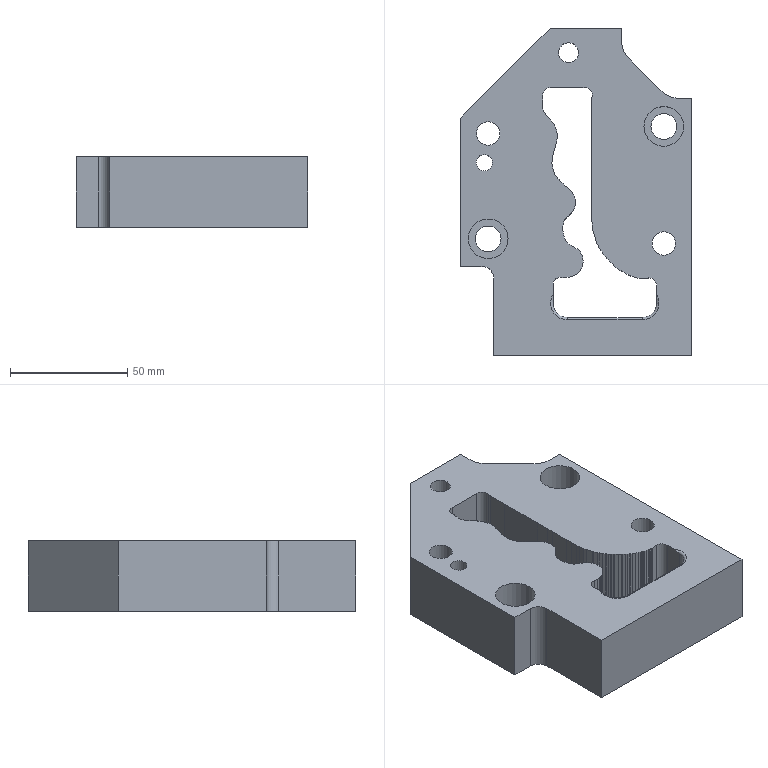Part | STEP file | 1 solid | 205 faces | box 99 x 140 x 30 mm | volume 280871 mm3 | plane 182 | cylinder 21 | torus 2 | commonest cylinder face diameters 6.28 x4 10 x3 11.72 x3 11 x2 12.28 x2 17 x2